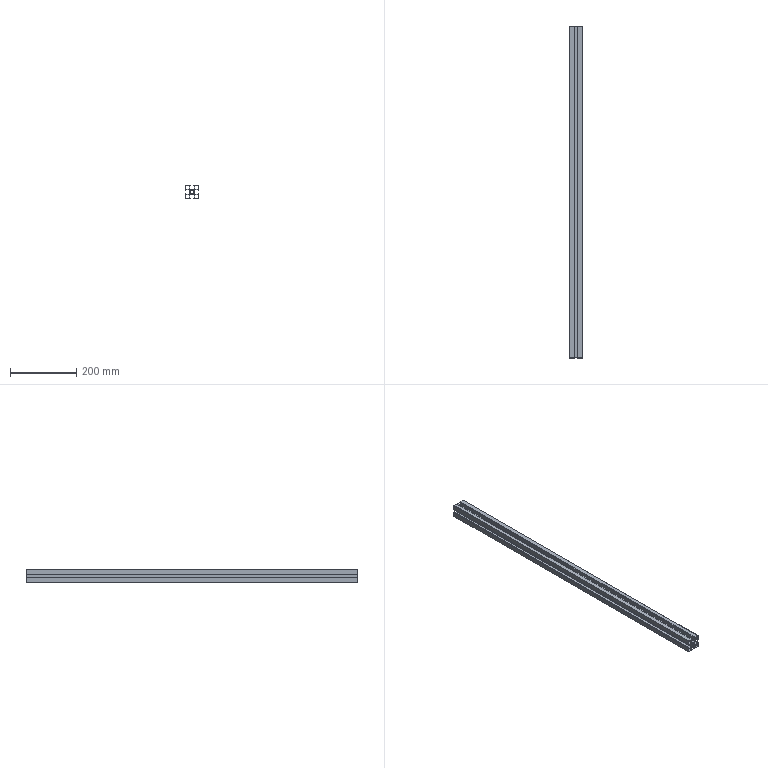Part | SolidWorks | features MirrorPattern 2, Extrusion 1 | 1 solid | 85 faces | box 40 x 1000 x 40 mm | volume 260790 mm3 | plane 70 | cylinder 15 | commonest cylinder face diameters 2 x6 10.6 x5 1 x4